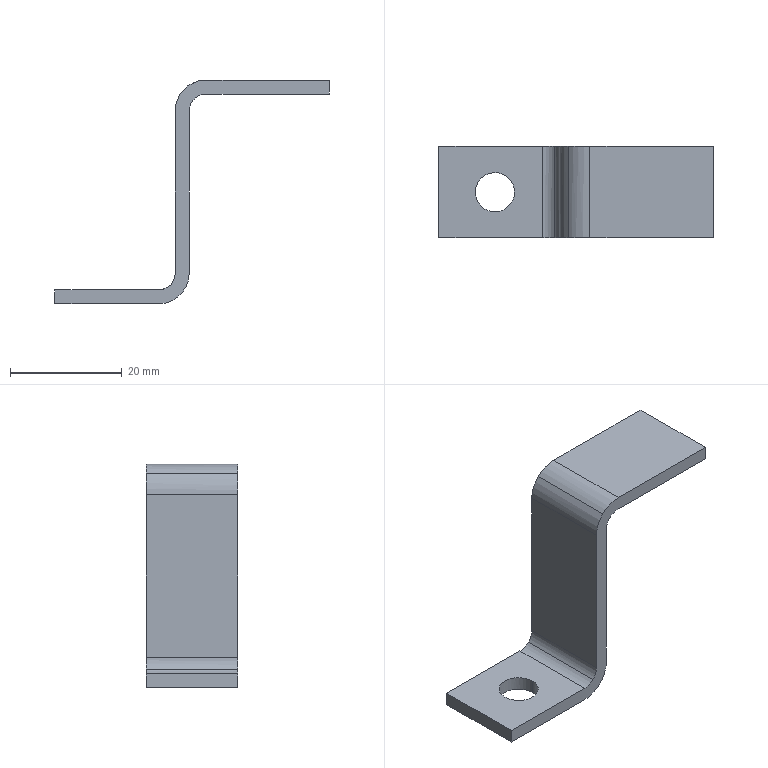Part | NX | features BREP 1 | 1 solid | 18 faces | box 49 x 16.34 x 40.003 mm | volume 3288 mm3 | plane 10 | cylinder 8 | commonest cylinder face diameters 6 x3 11 x3 7 x2
STEP:
#1=CARTESIAN_POINT('',(797.08,601.,1448.47));
#2=VERTEX_POINT('',#1);
#3=CARTESIAN_POINT('',(797.08,601.,1445.97));
#4=VERTEX_POINT('',#3);
#5=CARTESIAN_POINT('',(797.08,601.,1445.97));
#6=DIRECTION('',(0.,0.,1.));
#7=VECTOR('',#6,1000.);
#8=LINE('',#5,#7);
#9=EDGE_CURVE('',#2,#4,#8,.F.);
#10=ORIENTED_EDGE('',*,*,#9,.T.);
#11=CARTESIAN_POINT('',(790.08,601.,1445.97));
#12=VERTEX_POINT('',#11);
#13=CARTESIAN_POINT('',(790.08,601.,1445.97));
#14=CARTESIAN_POINT('',(790.08,600.633,1445.97));
#15=CARTESIAN_POINT('',(790.128,600.267,1445.97));
#16=CARTESIAN_POINT('',(790.224,599.909,1445.97));
#17=CARTESIAN_POINT('',(790.508,599.226,1445.97));
#18=CARTESIAN_POINT('',(790.957,598.639,1445.97));
#19=CARTESIAN_POINT('',(791.22,598.376,1445.97));
#20=CARTESIAN_POINT('',(791.807,597.927,1445.97));
#21=CARTESIAN_POINT('',(792.49,597.644,1445.97));
#22=CARTESIAN_POINT('',(792.848,597.548,1445.97));
#23=CARTESIAN_POINT('',(793.581,597.452,1445.97));
#24=CARTESIAN_POINT('',(794.314,597.548,1445.97));
#25=CARTESIAN_POINT('',(794.673,597.644,1445.97));
#26=CARTESIAN_POINT('',(795.356,597.928,1445.97));
#27=CARTESIAN_POINT('',(795.942,598.378,1445.97));
#28=CARTESIAN_POINT('',(796.204,598.641,1445.97));
#29=CARTESIAN_POINT('',(796.653,599.227,1445.97));
#30=CARTESIAN_POINT('',(796.936,599.91,1445.97));
#31=CARTESIAN_POINT('',(797.032,600.268,1445.97));
#32=CARTESIAN_POINT('',(797.08,600.634,1445.97));
#33=CARTESIAN_POINT('',(797.08,601.,1445.97));
#34=B_SPLINE_CURVE_WITH_KNOTS('',5,(#13,#14,#15,#16,#17,#18,#19,#20,#21,#22,#23,#24,#25,#26,#27,#28,#29,#30,#31,#32,#33),.UNSPECIFIED.,.F.,.F.,(6,3,3,3,3,3,6),(0.,2.592,5.185,7.777,10.369,12.961,15.55),.UNSPECIFIED.);
#35=EDGE_CURVE('',#12,#4,#34,.T.);
#36=ORIENTED_EDGE('',*,*,#35,.F.);
#37=CARTESIAN_POINT('',(790.08,601.,1448.47));
#38=VERTEX_POINT('',#37);
#39=CARTESIAN_POINT('',(790.08,601.,1445.97));
#40=DIRECTION('',(0.,0.,1.));
#41=VECTOR('',#40,1000.);
#42=LINE('',#39,#41);
#43=EDGE_CURVE('',#38,#12,#42,.F.);
#44=ORIENTED_EDGE('',*,*,#43,.F.);
#45=CARTESIAN_POINT('',(790.08,601.,1448.47));
#46=CARTESIAN_POINT('',(790.08,600.633,1448.47));
#47=CARTESIAN_POINT('',(790.128,600.267,1448.47));
#48=CARTESIAN_POINT('',(790.224,599.909,1448.47));
#49=CARTESIAN_POINT('',(790.508,599.226,1448.47));
#50=CARTESIAN_POINT('',(790.957,598.639,1448.47));
#51=CARTESIAN_POINT('',(791.22,598.376,1448.47));
#52=CARTESIAN_POINT('',(791.807,597.927,1448.47));
#53=CARTESIAN_POINT('',(792.49,597.644,1448.47));
#54=CARTESIAN_POINT('',(792.848,597.548,1448.47));
#55=CARTESIAN_POINT('',(793.581,597.452,1448.47));
#56=CARTESIAN_POINT('',(794.314,597.548,1448.47));
#57=CARTESIAN_POINT('',(794.673,597.644,1448.47));
#58=CARTESIAN_POINT('',(795.356,597.928,1448.47));
#59=CARTESIAN_POINT('',(795.942,598.378,1448.47));
#60=CARTESIAN_POINT('',(796.204,598.641,1448.47));
#61=CARTESIAN_POINT('',(796.653,599.227,1448.47));
#62=CARTESIAN_POINT('',(796.936,599.91,1448.47));
#63=CARTESIAN_POINT('',(797.032,600.268,1448.47));
#64=CARTESIAN_POINT('',(797.08,600.634,1448.47));
#65=CARTESIAN_POINT('',(797.08,601.,1448.47));
#66=B_SPLINE_CURVE_WITH_KNOTS('',5,(#45,#46,#47,#48,#49,#50,#51,#52,#53,#54,#55,#56,#57,#58,#59,#60,#61,#62,#63,#64,#65),.UNSPECIFIED.,.F.,.F.,(6,3,3,3,3,3,6),(0.,2.592,5.185,7.777,10.369,12.961,15.55),.UNSPECIFIED.);
#67=EDGE_CURVE('',#38,#2,#66,.T.);
#68=ORIENTED_EDGE('',*,*,#67,.T.);
#69=EDGE_LOOP('',(#10,#36,#44,#68));
#70=FACE_BOUND('',#69,.T.);
#71=CARTESIAN_POINT('',(793.58,601.,1445.97));
#72=DIRECTION('',(0.,0.,1.));
#73=DIRECTION('',(-1.,0.,0.));
#74=AXIS2_PLACEMENT_3D('',#71,#72,#73);
#75=CYLINDRICAL_SURFACE('',#74,3.5);
#76=ADVANCED_FACE('',(#70),#75,.F.);
#77=ORIENTED_EDGE('',*,*,#43,.T.);
#78=CARTESIAN_POINT('',(797.08,601.,1445.97));
#79=CARTESIAN_POINT('',(797.08,601.367,1445.97));
#80=CARTESIAN_POINT('',(797.032,601.733,1445.97));
#81=CARTESIAN_POINT('',(796.936,602.091,1445.97));
#82=CARTESIAN_POINT('',(796.652,602.774,1445.97));
#83=CARTESIAN_POINT('',(796.203,603.361,1445.97));
#84=CARTESIAN_POINT('',(795.94,603.624,1445.97));
#85=CARTESIAN_POINT('',(795.353,604.073,1445.97));
#86=CARTESIAN_POINT('',(794.67,604.356,1445.97));
#87=CARTESIAN_POINT('',(794.312,604.452,1445.97));
#88=CARTESIAN_POINT('',(793.579,604.548,1445.97));
#89=CARTESIAN_POINT('',(792.846,604.452,1445.97));
#90=CARTESIAN_POINT('',(792.487,604.356,1445.97));
#91=CARTESIAN_POINT('',(791.804,604.072,1445.97));
#92=CARTESIAN_POINT('',(791.218,603.622,1445.97));
#93=CARTESIAN_POINT('',(790.956,603.359,1445.97));
#94=CARTESIAN_POINT('',(790.507,602.773,1445.97));
#95=CARTESIAN_POINT('',(790.224,602.09,1445.97));
#96=CARTESIAN_POINT('',(790.128,601.732,1445.97));
#97=CARTESIAN_POINT('',(790.08,601.366,1445.97));
#98=CARTESIAN_POINT('',(790.08,601.,1445.97));
#99=B_SPLINE_CURVE_WITH_KNOTS('',5,(#78,#79,#80,#81,#82,#83,#84,#85,#86,#87,#88,#89,#90,#91,#92,#93,#94,#95,#96,#97,#98),.UNSPECIFIED.,.F.,.F.,(6,3,3,3,3,3,6),(0.,2.592,5.185,7.777,10.369,12.961,15.55),.UNSPECIFIED.);
#100=EDGE_CURVE('',#4,#12,#99,.T.);
#101=ORIENTED_EDGE('',*,*,#100,.F.);
#102=ORIENTED_EDGE('',*,*,#9,.F.);
#103=CARTESIAN_POINT('',(790.08,601.,1448.47));
#104=CARTESIAN_POINT('',(790.08,601.919,1448.47));
#105=CARTESIAN_POINT('',(790.837,603.74,1448.47));
#106=CARTESIAN_POINT('',(793.58,604.88,1448.47));
#107=CARTESIAN_POINT('',(796.323,603.74,1448.47));
#108=CARTESIAN_POINT('',(797.08,601.92,1448.47));
#109=CARTESIAN_POINT('',(797.08,601.,1448.47));
#110=B_SPLINE_CURVE_WITH_KNOTS('',3,(#103,#104,#105,#106,#107,#108,#109),.UNSPECIFIED.,.F.,.F.,(4,1,1,1,4),(0.,0.25,0.5,0.75,1.),.UNSPECIFIED.);
#111=EDGE_CURVE('',#38,#2,#110,.T.);
#112=ORIENTED_EDGE('',*,*,#111,.F.);
#113=EDGE_LOOP('',(#77,#101,#102,#112));
#114=FACE_BOUND('',#113,.T.);
#115=CARTESIAN_POINT('',(793.58,601.,1445.97));
#116=DIRECTION('',(0.,0.,1.));
#117=DIRECTION('',(1.,0.,0.));
#118=AXIS2_PLACEMENT_3D('',#115,#116,#117);
#119=CYLINDRICAL_SURFACE('',#118,3.5);
#120=ADVANCED_FACE('',(#114),#119,.F.);
#121=CARTESIAN_POINT('',(802.08,592.83,1445.97));
#122=VERTEX_POINT('',#121);
#123=CARTESIAN_POINT('',(783.58,592.83,1445.97));
#124=VERTEX_POINT('',#123);
#125=CARTESIAN_POINT('',(792.83,592.83,1445.97));
#126=DIRECTION('',(-1.,0.,0.));
#127=VECTOR('',#126,1000.);
#128=LINE('',#125,#127);
#129=EDGE_CURVE('',#122,#124,#128,.T.);
#130=ORIENTED_EDGE('',*,*,#129,.F.);
#131=CARTESIAN_POINT('',(807.58,592.83,1451.47));
#132=VERTEX_POINT('',#131);
#133=CARTESIAN_POINT('',(802.08,592.83,1451.47));
#134=DIRECTION('',(0.,1.,0.));
#135=DIRECTION('',(1.,0.,0.));
#136=AXIS2_PLACEMENT_3D('',#133,#134,#135);
#137=CIRCLE('',#136,5.5);
#138=EDGE_CURVE('',#132,#122,#137,.T.);
#139=ORIENTED_EDGE('',*,*,#138,.F.);
#140=CARTESIAN_POINT('',(807.58,592.83,1480.473));
#141=VERTEX_POINT('',#140);
#142=CARTESIAN_POINT('',(807.58,592.83,1465.971));
#143=DIRECTION('',(0.,0.,-1.));
#144=VECTOR('',#143,1000.);
#145=LINE('',#142,#144);
#146=EDGE_CURVE('',#141,#132,#145,.T.);
#147=ORIENTED_EDGE('',*,*,#146,.F.);
#148=CARTESIAN_POINT('',(810.58,592.83,1483.473));
#149=VERTEX_POINT('',#148);
#150=CARTESIAN_POINT('',(810.58,592.83,1480.473));
#151=DIRECTION('',(0.,1.,0.));
#152=DIRECTION('',(1.,0.,0.));
#153=AXIS2_PLACEMENT_3D('',#150,#151,#152);
#154=CIRCLE('',#153,3.);
#155=EDGE_CURVE('',#141,#149,#154,.T.);
#156=ORIENTED_EDGE('',*,*,#155,.T.);
#157=CARTESIAN_POINT('',(832.58,592.83,1483.473));
#158=VERTEX_POINT('',#157);
#159=CARTESIAN_POINT('',(821.58,592.83,1483.473));
#160=DIRECTION('',(-1.,0.,0.));
#161=VECTOR('',#160,1000.);
#162=LINE('',#159,#161);
#163=EDGE_CURVE('',#158,#149,#162,.T.);
#164=ORIENTED_EDGE('',*,*,#163,.F.);
#165=CARTESIAN_POINT('',(832.58,592.83,1485.973));
#166=VERTEX_POINT('',#165);
#167=CARTESIAN_POINT('',(832.58,592.83,1484.723));
#168=DIRECTION('',(0.,0.,-1.));
#169=VECTOR('',#168,1000.);
#170=LINE('',#167,#169);
#171=EDGE_CURVE('',#166,#158,#170,.T.);
#172=ORIENTED_EDGE('',*,*,#171,.F.);
#173=CARTESIAN_POINT('',(810.58,592.83,1485.973));
#174=VERTEX_POINT('',#173);
#175=CARTESIAN_POINT('',(821.58,592.83,1485.973));
#176=DIRECTION('',(-1.,0.,0.));
#177=VECTOR('',#176,1000.);
#178=LINE('',#175,#177);
#179=EDGE_CURVE('',#166,#174,#178,.T.);
#180=ORIENTED_EDGE('',*,*,#179,.T.);
#181=CARTESIAN_POINT('',(806.691,592.83,1484.362));
#182=VERTEX_POINT('',#181);
#183=CARTESIAN_POINT('',(810.58,592.83,1485.973));
#184=CARTESIAN_POINT('',(809.136,592.83,1485.973));
#185=CARTESIAN_POINT('',(807.713,592.83,1485.384));
#186=CARTESIAN_POINT('',(806.691,592.83,1484.362));
#187=B_SPLINE_CURVE_WITH_KNOTS('',3,(#183,#184,#185,#186),.UNSPECIFIED.,.F.,.F.,(4,4),(0.,1.),.UNSPECIFIED.);
#188=EDGE_CURVE('',#174,#182,#187,.T.);
#189=ORIENTED_EDGE('',*,*,#188,.T.);
#190=CARTESIAN_POINT('',(805.08,592.83,1480.473));
#191=VERTEX_POINT('',#190);
#192=CARTESIAN_POINT('',(806.691,592.83,1484.362));
#193=CARTESIAN_POINT('',(805.67,592.83,1483.341));
#194=CARTESIAN_POINT('',(805.08,592.83,1481.918));
#195=CARTESIAN_POINT('',(805.08,592.83,1480.473));
#196=B_SPLINE_CURVE_WITH_KNOTS('',3,(#192,#193,#194,#195),.UNSPECIFIED.,.F.,.F.,(4,4),(0.,1.),.UNSPECIFIED.);
#197=EDGE_CURVE('',#182,#191,#196,.T.);
#198=ORIENTED_EDGE('',*,*,#197,.T.);
#199=CARTESIAN_POINT('',(805.08,592.83,1451.47));
#200=VERTEX_POINT('',#199);
#201=CARTESIAN_POINT('',(805.08,592.83,1465.971));
#202=DIRECTION('',(0.,0.,-1.));
#203=VECTOR('',#202,1000.);
#204=LINE('',#201,#203);
#205=EDGE_CURVE('',#191,#200,#204,.T.);
#206=ORIENTED_EDGE('',*,*,#205,.T.);
#207=CARTESIAN_POINT('',(804.201,592.83,1449.349));
#208=VERTEX_POINT('',#207);
#209=CARTESIAN_POINT('',(805.08,592.83,1451.47));
#210=CARTESIAN_POINT('',(805.08,592.83,1450.683));
#211=CARTESIAN_POINT('',(804.759,592.83,1449.906));
#212=CARTESIAN_POINT('',(804.201,592.83,1449.349));
#213=B_SPLINE_CURVE_WITH_KNOTS('',3,(#209,#210,#211,#212),.UNSPECIFIED.,.F.,.F.,(4,4),(0.,1.),.UNSPECIFIED.);
#214=EDGE_CURVE('',#200,#208,#213,.T.);
#215=ORIENTED_EDGE('',*,*,#214,.T.);
#216=CARTESIAN_POINT('',(802.08,592.83,1448.47));
#217=VERTEX_POINT('',#216);
#218=CARTESIAN_POINT('',(804.201,592.83,1449.349));
#219=CARTESIAN_POINT('',(803.645,592.83,1448.792));
#220=CARTESIAN_POINT('',(802.869,592.83,1448.47));
#221=CARTESIAN_POINT('',(802.08,592.83,1448.47));
#222=B_SPLINE_CURVE_WITH_KNOTS('',3,(#218,#219,#220,#221),.UNSPECIFIED.,.F.,.F.,(4,4),(0.,1.),.UNSPECIFIED.);
#223=EDGE_CURVE('',#208,#217,#222,.T.);
#224=ORIENTED_EDGE('',*,*,#223,.T.);
#225=CARTESIAN_POINT('',(783.58,592.83,1448.47));
#226=VERTEX_POINT('',#225);
#227=CARTESIAN_POINT('',(792.83,592.83,1448.47));
#228=DIRECTION('',(-1.,0.,0.));
#229=VECTOR('',#228,1000.);
#230=LINE('',#227,#229);
#231=EDGE_CURVE('',#217,#226,#230,.T.);
#232=ORIENTED_EDGE('',*,*,#231,.T.);
#233=CARTESIAN_POINT('',(783.58,592.83,1447.22));
#234=DIRECTION('',(0.,0.,-1.));
#235=VECTOR('',#234,1000.);
#236=LINE('',#233,#235);
#237=EDGE_CURVE('',#226,#124,#236,.T.);
#238=ORIENTED_EDGE('',*,*,#237,.T.);
#239=EDGE_LOOP('',(#130,#139,#147,#156,#164,#172,#180,#189,#198,#206,#215,#224,#232,#238));
#240=FACE_BOUND('',#239,.T.);
#241=CARTESIAN_POINT('',(804.34,592.83,1470.98));
#242=DIRECTION('',(0.,-1.,0.));
#243=DIRECTION('',(0.,0.,1.));
#244=AXIS2_PLACEMENT_3D('',#241,#242,#243);
#245=PLANE('',#244);
#246=ADVANCED_FACE('',(#240),#245,.T.);
#247=CARTESIAN_POINT('',(832.58,609.17,1485.973));
#248=VERTEX_POINT('',#247);
#249=CARTESIAN_POINT('',(810.58,609.17,1485.973));
#250=VERTEX_POINT('',#249);
#251=CARTESIAN_POINT('',(821.58,609.17,1485.973));
#252=DIRECTION('',(-1.,0.,0.));
#253=VECTOR('',#252,1000.);
#254=LINE('',#251,#253);
#255=EDGE_CURVE('',#248,#250,#254,.T.);
#256=ORIENTED_EDGE('',*,*,#255,.T.);
#257=CARTESIAN_POINT('',(810.58,601.,1485.973));
#258=DIRECTION('',(0.,1.,0.));
#259=VECTOR('',#258,1000.);
#260=LINE('',#257,#259);
#261=EDGE_CURVE('',#174,#250,#260,.T.);
#262=ORIENTED_EDGE('',*,*,#261,.F.);
#263=ORIENTED_EDGE('',*,*,#179,.F.);
#264=CARTESIAN_POINT('',(832.58,601.,1485.973));
#265=DIRECTION('',(0.,1.,0.));
#266=VECTOR('',#265,1000.);
#267=LINE('',#264,#266);
#268=EDGE_CURVE('',#166,#248,#267,.T.);
#269=ORIENTED_EDGE('',*,*,#268,.T.);
#270=EDGE_LOOP('',(#256,#262,#263,#269));
#271=FACE_BOUND('',#270,.T.);
#272=CARTESIAN_POINT('',(832.58,601.,1485.973));
#273=DIRECTION('',(0.,0.,-1.));
#274=DIRECTION('',(-1.,0.,0.));
#275=AXIS2_PLACEMENT_3D('',#272,#273,#274);
#276=PLANE('',#275);
#277=ADVANCED_FACE('',(#271),#276,.F.);
#278=CARTESIAN_POINT('',(806.691,609.17,1484.362));
#279=VERTEX_POINT('',#278);
#280=CARTESIAN_POINT('',(806.691,601.,1484.362));
#281=DIRECTION('',(0.,1.,0.));
#282=VECTOR('',#281,1000.);
#283=LINE('',#280,#282);
#284=EDGE_CURVE('',#182,#279,#283,.T.);
#285=ORIENTED_EDGE('',*,*,#284,.F.);
#286=ORIENTED_EDGE('',*,*,#188,.F.);
#287=ORIENTED_EDGE('',*,*,#261,.T.);
#288=CARTESIAN_POINT('',(810.58,609.17,1480.473));
#289=DIRECTION('',(0.,-1.,0.));
#290=DIRECTION('',(1.,0.,0.));
#291=AXIS2_PLACEMENT_3D('',#288,#289,#290);
#292=CIRCLE('',#291,5.5);
#293=EDGE_CURVE('',#250,#279,#292,.T.);
#294=ORIENTED_EDGE('',*,*,#293,.T.);
#295=EDGE_LOOP('',(#285,#286,#287,#294));
#296=FACE_BOUND('',#295,.T.);
#297=CARTESIAN_POINT('',(810.58,601.,1480.473));
#298=DIRECTION('',(0.,1.,0.));
#299=DIRECTION('',(-0.7071,0.,0.7071));
#300=AXIS2_PLACEMENT_3D('',#297,#298,#299);
#301=CYLINDRICAL_SURFACE('',#300,5.5);
#302=ADVANCED_FACE('',(#296),#301,.T.);
#303=ORIENTED_EDGE('',*,*,#284,.T.);
#304=CARTESIAN_POINT('',(805.08,609.17,1480.473));
#305=VERTEX_POINT('',#304);
#306=CARTESIAN_POINT('',(810.58,609.17,1480.473));
#307=DIRECTION('',(0.,-1.,0.));
#308=DIRECTION('',(1.,0.,0.));
#309=AXIS2_PLACEMENT_3D('',#306,#307,#308);
#310=CIRCLE('',#309,5.5);
#311=EDGE_CURVE('',#279,#305,#310,.T.);
#312=ORIENTED_EDGE('',*,*,#311,.T.);
#313=CARTESIAN_POINT('',(805.08,601.,1480.473));
#314=DIRECTION('',(0.,1.,0.));
#315=VECTOR('',#314,1000.);
#316=LINE('',#313,#315);
#317=EDGE_CURVE('',#191,#305,#316,.T.);
#318=ORIENTED_EDGE('',*,*,#317,.F.);
#319=ORIENTED_EDGE('',*,*,#197,.F.);
#320=EDGE_LOOP('',(#303,#312,#318,#319));
#321=FACE_BOUND('',#320,.T.);
#322=CARTESIAN_POINT('',(810.58,601.,1480.473));
#323=DIRECTION('',(0.,1.,0.));
#324=DIRECTION('',(0.7071,0.,-0.7071));
#325=AXIS2_PLACEMENT_3D('',#322,#323,#324);
#326=CYLINDRICAL_SURFACE('',#325,5.5);
#327=ADVANCED_FACE('',(#321),#326,.T.);
#328=CARTESIAN_POINT('',(805.08,609.17,1451.47));
#329=VERTEX_POINT('',#328);
#330=CARTESIAN_POINT('',(805.08,609.17,1465.971));
#331=DIRECTION('',(0.,0.,-1.));
#332=VECTOR('',#331,1000.);
#333=LINE('',#330,#332);
#334=EDGE_CURVE('',#305,#329,#333,.T.);
#335=ORIENTED_EDGE('',*,*,#334,.T.);
#336=CARTESIAN_POINT('',(805.08,601.,1451.47));
#337=DIRECTION('',(0.,1.,0.));
#338=VECTOR('',#337,1000.);
#339=LINE('',#336,#338);
#340=EDGE_CURVE('',#200,#329,#339,.T.);
#341=ORIENTED_EDGE('',*,*,#340,.F.);
#342=ORIENTED_EDGE('',*,*,#205,.F.);
#343=ORIENTED_EDGE('',*,*,#317,.T.);
#344=EDGE_LOOP('',(#335,#341,#342,#343));
#345=FACE_BOUND('',#344,.T.);
#346=CARTESIAN_POINT('',(805.08,601.,1483.473));
#347=DIRECTION('',(1.,0.,0.));
#348=DIRECTION('',(0.,0.,-1.));
#349=AXIS2_PLACEMENT_3D('',#346,#347,#348);
#350=PLANE('',#349);
#351=ADVANCED_FACE('',(#345),#350,.F.);
#352=ORIENTED_EDGE('',*,*,#214,.F.);
#353=ORIENTED_EDGE('',*,*,#340,.T.);
#354=CARTESIAN_POINT('',(804.201,609.17,1449.349));
#355=VERTEX_POINT('',#354);
#356=CARTESIAN_POINT('',(802.08,609.17,1451.47));
#357=DIRECTION('',(0.,-1.,0.));
#358=DIRECTION('',(1.,0.,0.));
#359=AXIS2_PLACEMENT_3D('',#356,#357,#358);
#360=CIRCLE('',#359,3.);
#361=EDGE_CURVE('',#355,#329,#360,.T.);
#362=ORIENTED_EDGE('',*,*,#361,.F.);
#363=CARTESIAN_POINT('',(804.201,601.,1449.349));
#364=DIRECTION('',(0.,1.,0.));
#365=VECTOR('',#364,1000.);
#366=LINE('',#363,#365);
#367=EDGE_CURVE('',#208,#355,#366,.T.);
#368=ORIENTED_EDGE('',*,*,#367,.F.);
#369=EDGE_LOOP('',(#352,#353,#362,#368));
#370=FACE_BOUND('',#369,.T.);
#371=CARTESIAN_POINT('',(802.08,601.,1451.47));
#372=DIRECTION('',(0.,1.,0.));
#373=DIRECTION('',(-0.7071,0.,0.7071));
#374=AXIS2_PLACEMENT_3D('',#371,#372,#373);
#375=CYLINDRICAL_SURFACE('',#374,3.);
#376=ADVANCED_FACE('',(#370),#375,.F.);
#377=CARTESIAN_POINT('',(802.08,609.17,1448.47));
#378=VERTEX_POINT('',#377);
#379=CARTESIAN_POINT('',(802.08,609.17,1451.47));
#380=DIRECTION('',(0.,-1.,0.));
#381=DIRECTION('',(1.,0.,0.));
#382=AXIS2_PLACEMENT_3D('',#379,#380,#381);
#383=CIRCLE('',#382,3.);
#384=EDGE_CURVE('',#378,#355,#383,.T.);
#385=ORIENTED_EDGE('',*,*,#384,.F.);
#386=CARTESIAN_POINT('',(802.08,601.,1448.47));
#387=DIRECTION('',(0.,1.,0.));
#388=VECTOR('',#387,1000.);
#389=LINE('',#386,#388);
#390=EDGE_CURVE('',#217,#378,#389,.T.);
#391=ORIENTED_EDGE('',*,*,#390,.F.);
#392=ORIENTED_EDGE('',*,*,#223,.F.);
#393=ORIENTED_EDGE('',*,*,#367,.T.);
#394=EDGE_LOOP('',(#385,#391,#392,#393));
#395=FACE_BOUND('',#394,.T.);
#396=CARTESIAN_POINT('',(802.08,601.,1451.47));
#397=DIRECTION('',(0.,1.,0.));
#398=DIRECTION('',(0.7071,0.,-0.7071));
#399=AXIS2_PLACEMENT_3D('',#396,#397,#398);
#400=CYLINDRICAL_SURFACE('',#399,3.);
#401=ADVANCED_FACE('',(#395),#400,.F.);
#402=ORIENTED_EDGE('',*,*,#67,.F.);
#403=ORIENTED_EDGE('',*,*,#111,.T.);
#404=EDGE_LOOP('',(#402,#403));
#405=FACE_BOUND('',#404,.T.);
#406=CARTESIAN_POINT('',(783.58,609.17,1448.47));
#407=VERTEX_POINT('',#406);
#408=CARTESIAN_POINT('',(792.83,609.17,1448.47));
#409=DIRECTION('',(-1.,0.,0.));
#410=VECTOR('',#409,1000.);
#411=LINE('',#408,#410);
#412=EDGE_CURVE('',#378,#407,#411,.T.);
#413=ORIENTED_EDGE('',*,*,#412,.T.);
#414=CARTESIAN_POINT('',(783.58,601.,1448.47));
#415=DIRECTION('',(0.,1.,0.));
#416=VECTOR('',#415,1000.);
#417=LINE('',#414,#416);
#418=EDGE_CURVE('',#226,#407,#417,.T.);
#419=ORIENTED_EDGE('',*,*,#418,.F.);
#420=ORIENTED_EDGE('',*,*,#231,.F.);
#421=ORIENTED_EDGE('',*,*,#390,.T.);
#422=EDGE_LOOP('',(#413,#419,#420,#421));
#423=FACE_BOUND('',#422,.T.);
#424=CARTESIAN_POINT('',(807.58,601.,1448.47));
#425=DIRECTION('',(0.,0.,-1.));
#426=DIRECTION('',(-1.,0.,0.));
#427=AXIS2_PLACEMENT_3D('',#424,#425,#426);
#428=PLANE('',#427);
#429=ADVANCED_FACE('',(#405,#423),#428,.F.);
#430=CARTESIAN_POINT('',(783.58,609.17,1445.97));
#431=VERTEX_POINT('',#430);
#432=CARTESIAN_POINT('',(783.58,609.17,1447.22));
#433=DIRECTION('',(0.,0.,-1.));
#434=VECTOR('',#433,1000.);
#435=LINE('',#432,#434);
#436=EDGE_CURVE('',#407,#431,#435,.T.);
#437=ORIENTED_EDGE('',*,*,#436,.T.);
#438=CARTESIAN_POINT('',(783.58,601.,1445.97));
#439=DIRECTION('',(0.,1.,0.));
#440=VECTOR('',#439,1000.);
#441=LINE('',#438,#440);
#442=EDGE_CURVE('',#124,#431,#441,.T.);
#443=ORIENTED_EDGE('',*,*,#442,.F.);
#444=ORIENTED_EDGE('',*,*,#237,.F.);
#445=ORIENTED_EDGE('',*,*,#418,.T.);
#446=EDGE_LOOP('',(#437,#443,#444,#445));
#447=FACE_BOUND('',#446,.T.);
#448=CARTESIAN_POINT('',(783.58,601.,1445.97));
#449=DIRECTION('',(1.,0.,0.));
#450=DIRECTION('',(0.,1.,0.));
#451=AXIS2_PLACEMENT_3D('',#448,#449,#450);
#452=PLANE('',#451);
#453=ADVANCED_FACE('',(#447),#452,.F.);
#454=ORIENTED_EDGE('',*,*,#100,.T.);
#455=ORIENTED_EDGE('',*,*,#35,.T.);
#456=EDGE_LOOP('',(#454,#455));
#457=FACE_BOUND('',#456,.T.);
#458=CARTESIAN_POINT('',(802.08,609.17,1445.97));
#459=VERTEX_POINT('',#458);
#460=CARTESIAN_POINT('',(802.08,601.,1445.97));
#461=DIRECTION('',(0.,1.,0.));
#462=VECTOR('',#461,1000.);
#463=LINE('',#460,#462);
#464=EDGE_CURVE('',#122,#459,#463,.T.);
#465=ORIENTED_EDGE('',*,*,#464,.F.);
#466=ORIENTED_EDGE('',*,*,#129,.T.);
#467=ORIENTED_EDGE('',*,*,#442,.T.);
#468=CARTESIAN_POINT('',(792.83,609.17,1445.97));
#469=DIRECTION('',(-1.,0.,0.));
#470=VECTOR('',#469,1000.);
#471=LINE('',#468,#470);
#472=EDGE_CURVE('',#459,#431,#471,.T.);
#473=ORIENTED_EDGE('',*,*,#472,.F.);
#474=EDGE_LOOP('',(#465,#466,#467,#473));
#475=FACE_BOUND('',#474,.T.);
#476=CARTESIAN_POINT('',(807.58,601.,1445.97));
#477=DIRECTION('',(0.,0.,-1.));
#478=DIRECTION('',(-1.,0.,0.));
#479=AXIS2_PLACEMENT_3D('',#476,#477,#478);
#480=PLANE('',#479);
#481=ADVANCED_FACE('',(#457,#475),#480,.T.);
#482=CARTESIAN_POINT('',(807.58,609.17,1451.47));
#483=VERTEX_POINT('',#482);
#484=CARTESIAN_POINT('',(807.58,601.,1451.47));
#485=DIRECTION('',(0.,1.,0.));
#486=VECTOR('',#485,1000.);
#487=LINE('',#484,#486);
#488=EDGE_CURVE('',#132,#483,#487,.T.);
#489=ORIENTED_EDGE('',*,*,#488,.F.);
#490=ORIENTED_EDGE('',*,*,#138,.T.);
#491=ORIENTED_EDGE('',*,*,#464,.T.);
#492=CARTESIAN_POINT('',(802.08,609.17,1451.47));
#493=DIRECTION('',(0.,-1.,0.));
#494=DIRECTION('',(1.,0.,0.));
#495=AXIS2_PLACEMENT_3D('',#492,#493,#494);
#496=CIRCLE('',#495,5.5);
#497=EDGE_CURVE('',#459,#483,#496,.T.);
#498=ORIENTED_EDGE('',*,*,#497,.T.);
#499=EDGE_LOOP('',(#489,#490,#491,#498));
#500=FACE_BOUND('',#499,.T.);
#501=CARTESIAN_POINT('',(802.08,601.,1451.47));
#502=DIRECTION('',(0.,1.,0.));
#503=DIRECTION('',(1.,0.,0.));
#504=AXIS2_PLACEMENT_3D('',#501,#502,#503);
#505=CYLINDRICAL_SURFACE('',#504,5.5);
#506=ADVANCED_FACE('',(#500),#505,.T.);
#507=CARTESIAN_POINT('',(807.58,609.17,1480.473));
#508=VERTEX_POINT('',#507);
#509=CARTESIAN_POINT('',(807.58,601.,1480.473));
#510=DIRECTION('',(0.,1.,0.));
#511=VECTOR('',#510,1000.);
#512=LINE('',#509,#511);
#513=EDGE_CURVE('',#141,#508,#512,.T.);
#514=ORIENTED_EDGE('',*,*,#513,.F.);
#515=ORIENTED_EDGE('',*,*,#146,.T.);
#516=ORIENTED_EDGE('',*,*,#488,.T.);
#517=CARTESIAN_POINT('',(807.58,609.17,1465.971));
#518=DIRECTION('',(0.,0.,-1.));
#519=VECTOR('',#518,1000.);
#520=LINE('',#517,#519);
#521=EDGE_CURVE('',#508,#483,#520,.T.);
#522=ORIENTED_EDGE('',*,*,#521,.F.);
#523=EDGE_LOOP('',(#514,#515,#516,#522));
#524=FACE_BOUND('',#523,.T.);
#525=CARTESIAN_POINT('',(807.58,601.,1483.473));
#526=DIRECTION('',(1.,0.,0.));
#527=DIRECTION('',(0.,0.,-1.));
#528=AXIS2_PLACEMENT_3D('',#525,#526,#527);
#529=PLANE('',#528);
#530=ADVANCED_FACE('',(#524),#529,.T.);
#531=CARTESIAN_POINT('',(810.58,609.17,1483.473));
#532=VERTEX_POINT('',#531);
#533=CARTESIAN_POINT('',(810.58,609.17,1480.473));
#534=DIRECTION('',(0.,-1.,0.));
#535=DIRECTION('',(1.,0.,0.));
#536=AXIS2_PLACEMENT_3D('',#533,#534,#535);
#537=CIRCLE('',#536,3.);
#538=EDGE_CURVE('',#532,#508,#537,.T.);
#539=ORIENTED_EDGE('',*,*,#538,.F.);
#540=CARTESIAN_POINT('',(810.58,601.,1483.473));
#541=DIRECTION('',(0.,1.,0.));
#542=VECTOR('',#541,1000.);
#543=LINE('',#540,#542);
#544=EDGE_CURVE('',#149,#532,#543,.T.);
#545=ORIENTED_EDGE('',*,*,#544,.F.);
#546=ORIENTED_EDGE('',*,*,#155,.F.);
#547=ORIENTED_EDGE('',*,*,#513,.T.);
#548=EDGE_LOOP('',(#539,#545,#546,#547));
#549=FACE_BOUND('',#548,.T.);
#550=CARTESIAN_POINT('',(810.58,601.,1480.473));
#551=DIRECTION('',(0.,1.,0.));
#552=DIRECTION('',(-1.,0.,0.));
#553=AXIS2_PLACEMENT_3D('',#550,#551,#552);
#554=CYLINDRICAL_SURFACE('',#553,3.);
#555=ADVANCED_FACE('',(#549),#554,.F.);
#556=CARTESIAN_POINT('',(832.58,609.17,1483.473));
#557=VERTEX_POINT('',#556);
#558=CARTESIAN_POINT('',(832.58,601.,1483.473));
#559=DIRECTION('',(0.,1.,0.));
#560=VECTOR('',#559,1000.);
#561=LINE('',#558,#560);
#562=EDGE_CURVE('',#158,#557,#561,.T.);
#563=ORIENTED_EDGE('',*,*,#562,.F.);
#564=ORIENTED_EDGE('',*,*,#163,.T.);
#565=ORIENTED_EDGE('',*,*,#544,.T.);
#566=CARTESIAN_POINT('',(821.58,609.17,1483.473));
#567=DIRECTION('',(-1.,0.,0.));
#568=VECTOR('',#567,1000.);
#569=LINE('',#566,#568);
#570=EDGE_CURVE('',#557,#532,#569,.T.);
#571=ORIENTED_EDGE('',*,*,#570,.F.);
#572=EDGE_LOOP('',(#563,#564,#565,#571));
#573=FACE_BOUND('',#572,.T.);
#574=CARTESIAN_POINT('',(832.58,601.,1483.473));
#575=DIRECTION('',(0.,0.,-1.));
#576=DIRECTION('',(-1.,0.,0.));
#577=AXIS2_PLACEMENT_3D('',#574,#575,#576);
#578=PLANE('',#577);
#579=ADVANCED_FACE('',(#573),#578,.T.);
#580=ORIENTED_EDGE('',*,*,#268,.F.);
#581=ORIENTED_EDGE('',*,*,#171,.T.);
#582=ORIENTED_EDGE('',*,*,#562,.T.);
#583=CARTESIAN_POINT('',(832.58,609.17,1484.723));
#584=DIRECTION('',(0.,0.,-1.));
#585=VECTOR('',#584,1000.);
#586=LINE('',#583,#585);
#587=EDGE_CURVE('',#248,#557,#586,.T.);
#588=ORIENTED_EDGE('',*,*,#587,.F.);
#589=EDGE_LOOP('',(#580,#581,#582,#588));
#590=FACE_BOUND('',#589,.T.);
#591=CARTESIAN_POINT('',(832.58,601.,1483.473));
#592=DIRECTION('',(1.,0.,0.));
#593=DIRECTION('',(0.,1.,0.));
#594=AXIS2_PLACEMENT_3D('',#591,#592,#593);
#595=PLANE('',#594);
#596=ADVANCED_FACE('',(#590),#595,.T.);
#597=ORIENTED_EDGE('',*,*,#587,.T.);
#598=ORIENTED_EDGE('',*,*,#570,.T.);
#599=ORIENTED_EDGE('',*,*,#538,.T.);
#600=ORIENTED_EDGE('',*,*,#521,.T.);
#601=ORIENTED_EDGE('',*,*,#497,.F.);
#602=ORIENTED_EDGE('',*,*,#472,.T.);
#603=ORIENTED_EDGE('',*,*,#436,.F.);
#604=ORIENTED_EDGE('',*,*,#412,.F.);
#605=ORIENTED_EDGE('',*,*,#384,.T.);
#606=ORIENTED_EDGE('',*,*,#361,.T.);
#607=ORIENTED_EDGE('',*,*,#334,.F.);
#608=ORIENTED_EDGE('',*,*,#311,.F.);
#609=ORIENTED_EDGE('',*,*,#293,.F.);
#610=ORIENTED_EDGE('',*,*,#255,.F.);
#611=EDGE_LOOP('',(#597,#598,#599,#600,#601,#602,#603,#604,#605,#606,#607,#608,#609,#610));
#612=FACE_BOUND('',#611,.T.);
#613=CARTESIAN_POINT('',(804.34,609.17,1470.98));
#614=DIRECTION('',(0.,-1.,0.));
#615=DIRECTION('',(0.,0.,1.));
#616=AXIS2_PLACEMENT_3D('',#613,#614,#615);
#617=PLANE('',#616);
#618=ADVANCED_FACE('',(#612),#617,.F.);
#619=CLOSED_SHELL('',(#76,#120,#246,#277,#302,#327,#351,#376,#401,#429,#453,#481,#506,#530,#555,#579,#596,#618));
#620=MANIFOLD_SOLID_BREP('',#619);
#621=(LENGTH_UNIT()NAMED_UNIT(*)SI_UNIT(.MILLI.,.METRE.));
#622=UNCERTAINTY_MEASURE_WITH_UNIT(LENGTH_MEASURE(0.0508),#621,'','');
#623=(NAMED_UNIT(*)PLANE_ANGLE_UNIT()SI_UNIT($,.RADIAN.));
#624=(NAMED_UNIT(*)SI_UNIT($,.STERADIAN.)SOLID_ANGLE_UNIT());
#625=(GEOMETRIC_REPRESENTATION_CONTEXT(3)GLOBAL_UNCERTAINTY_ASSIGNED_CONTEXT((#622))GLOBAL_UNIT_ASSIGNED_CONTEXT((#621,#623,#624))REPRESENTATION_CONTEXT('',''));
#626=ADVANCED_BREP_SHAPE_REPRESENTATION('',(#620),#625);